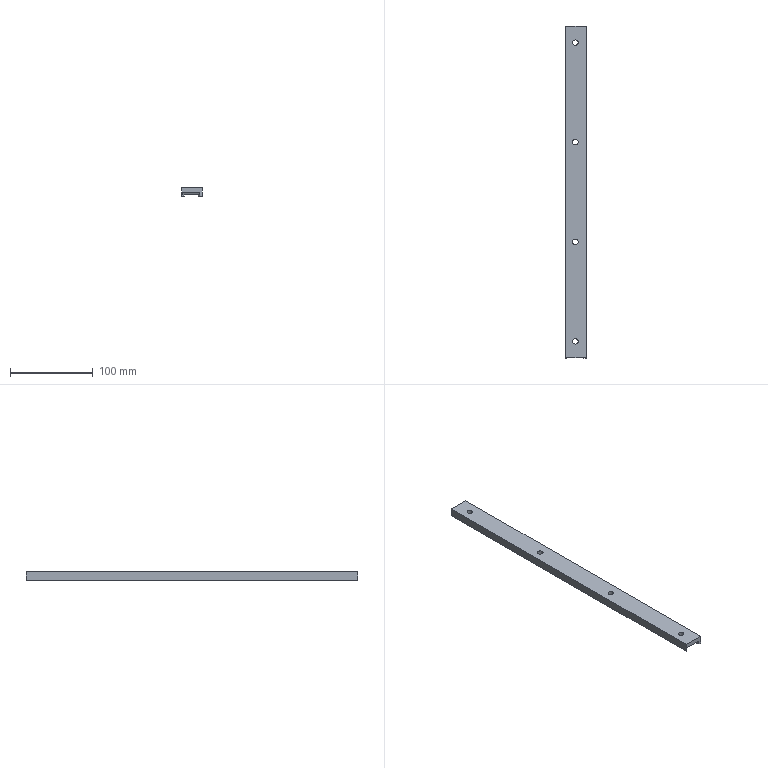Part | SolidWorks | features BaseBody 1 | 1 solid | 29 faces | box 24.5 x 400 x 10 mm | volume 79904 mm3 | plane 13 | cone 8 | cylinder 8 | commonest cylinder face diameters 6.6 x8
STEP:
#1=CARTESIAN_POINT('',(14.8,180.,-4.5));
#2=VERTEX_POINT('',#1);
#3=CARTESIAN_POINT('',(8.2,180.,-4.5));
#4=VERTEX_POINT('',#3);
#5=CARTESIAN_POINT('',(11.5,180.,-4.5));
#6=DIRECTION('',(0.,0.,-1.));
#7=DIRECTION('',(-1.,0.,0.));
#8=AXIS2_PLACEMENT_3D('',#5,#6,#7);
#9=CIRCLE('',#8,3.3);
#10=EDGE_CURVE('',#2,#4,#9,.T.);
#11=ORIENTED_EDGE('',*,*,#10,.F.);
#12=CARTESIAN_POINT('',(17.9,180.,-7.6));
#13=VERTEX_POINT('',#12);
#14=CARTESIAN_POINT('',(17.9,180.,-7.6));
#15=DIRECTION('',(0.7071,0.,-0.7071));
#16=VECTOR('',#15,1000.);
#17=LINE('',#14,#16);
#18=EDGE_CURVE('',#2,#13,#17,.T.);
#19=ORIENTED_EDGE('',*,*,#18,.T.);
#20=CARTESIAN_POINT('',(5.1,180.,-7.6));
#21=VERTEX_POINT('',#20);
#22=CARTESIAN_POINT('',(11.5,180.,-7.6));
#23=DIRECTION('',(0.,0.,-1.));
#24=DIRECTION('',(-1.,0.,0.));
#25=AXIS2_PLACEMENT_3D('',#22,#23,#24);
#26=CIRCLE('',#25,6.4);
#27=EDGE_CURVE('',#13,#21,#26,.T.);
#28=ORIENTED_EDGE('',*,*,#27,.T.);
#29=CARTESIAN_POINT('',(5.1,180.,-7.6));
#30=DIRECTION('',(-0.7071,0.,-0.7071));
#31=VECTOR('',#30,1000.);
#32=LINE('',#29,#31);
#33=EDGE_CURVE('',#4,#21,#32,.T.);
#34=ORIENTED_EDGE('',*,*,#33,.F.);
#35=EDGE_LOOP('',(#11,#19,#28,#34));
#36=FACE_OUTER_BOUND('',#35,.T.);
#37=CARTESIAN_POINT('',(11.5,180.,-7.6));
#38=DIRECTION('',(0.,0.,-1.));
#39=DIRECTION('',(-1.,0.,0.));
#40=AXIS2_PLACEMENT_3D('',#37,#38,#39);
#41=CONICAL_SURFACE('',#40,6.4,0.7854);
#42=ADVANCED_FACE('',(#36),#41,.F.);
#43=CARTESIAN_POINT('',(14.8,180.,0.));
#44=VERTEX_POINT('',#43);
#45=CARTESIAN_POINT('',(8.2,180.,0.));
#46=VERTEX_POINT('',#45);
#47=CARTESIAN_POINT('',(11.5,180.,0.));
#48=DIRECTION('',(0.,0.,-1.));
#49=DIRECTION('',(-1.,0.,0.));
#50=AXIS2_PLACEMENT_3D('',#47,#48,#49);
#51=CIRCLE('',#50,3.3);
#52=EDGE_CURVE('',#44,#46,#51,.T.);
#53=ORIENTED_EDGE('',*,*,#52,.F.);
#54=CARTESIAN_POINT('',(14.8,180.,-7.6));
#55=DIRECTION('',(0.,0.,-1.));
#56=VECTOR('',#55,1000.);
#57=LINE('',#54,#56);
#58=EDGE_CURVE('',#44,#2,#57,.T.);
#59=ORIENTED_EDGE('',*,*,#58,.T.);
#60=ORIENTED_EDGE('',*,*,#10,.T.);
#61=CARTESIAN_POINT('',(8.2,180.,-7.6));
#62=DIRECTION('',(0.,0.,-1.));
#63=VECTOR('',#62,1000.);
#64=LINE('',#61,#63);
#65=EDGE_CURVE('',#46,#4,#64,.T.);
#66=ORIENTED_EDGE('',*,*,#65,.F.);
#67=EDGE_LOOP('',(#53,#59,#60,#66));
#68=FACE_OUTER_BOUND('',#67,.T.);
#69=CARTESIAN_POINT('',(11.5,180.,-7.6));
#70=DIRECTION('',(0.,0.,-1.));
#71=DIRECTION('',(-1.,0.,0.));
#72=AXIS2_PLACEMENT_3D('',#69,#70,#71);
#73=CYLINDRICAL_SURFACE('',#72,3.3);
#74=ADVANCED_FACE('',(#68),#73,.F.);
#75=CARTESIAN_POINT('',(14.8,60.,-4.5));
#76=VERTEX_POINT('',#75);
#77=CARTESIAN_POINT('',(8.2,60.,-4.5));
#78=VERTEX_POINT('',#77);
#79=CARTESIAN_POINT('',(11.5,60.,-4.5));
#80=DIRECTION('',(0.,0.,-1.));
#81=DIRECTION('',(-1.,0.,0.));
#82=AXIS2_PLACEMENT_3D('',#79,#80,#81);
#83=CIRCLE('',#82,3.3);
#84=EDGE_CURVE('',#76,#78,#83,.T.);
#85=ORIENTED_EDGE('',*,*,#84,.F.);
#86=CARTESIAN_POINT('',(17.9,60.,-7.6));
#87=VERTEX_POINT('',#86);
#88=CARTESIAN_POINT('',(17.9,60.,-7.6));
#89=DIRECTION('',(0.7071,0.,-0.7071));
#90=VECTOR('',#89,1000.);
#91=LINE('',#88,#90);
#92=EDGE_CURVE('',#76,#87,#91,.T.);
#93=ORIENTED_EDGE('',*,*,#92,.T.);
#94=CARTESIAN_POINT('',(5.1,60.,-7.6));
#95=VERTEX_POINT('',#94);
#96=CARTESIAN_POINT('',(11.5,60.,-7.6));
#97=DIRECTION('',(0.,0.,-1.));
#98=DIRECTION('',(-1.,0.,0.));
#99=AXIS2_PLACEMENT_3D('',#96,#97,#98);
#100=CIRCLE('',#99,6.4);
#101=EDGE_CURVE('',#87,#95,#100,.T.);
#102=ORIENTED_EDGE('',*,*,#101,.T.);
#103=CARTESIAN_POINT('',(5.1,60.,-7.6));
#104=DIRECTION('',(-0.7071,0.,-0.7071));
#105=VECTOR('',#104,1000.);
#106=LINE('',#103,#105);
#107=EDGE_CURVE('',#78,#95,#106,.T.);
#108=ORIENTED_EDGE('',*,*,#107,.F.);
#109=EDGE_LOOP('',(#85,#93,#102,#108));
#110=FACE_OUTER_BOUND('',#109,.T.);
#111=CARTESIAN_POINT('',(11.5,60.,-7.6));
#112=DIRECTION('',(0.,0.,-1.));
#113=DIRECTION('',(-1.,0.,0.));
#114=AXIS2_PLACEMENT_3D('',#111,#112,#113);
#115=CONICAL_SURFACE('',#114,6.4,0.7854);
#116=ADVANCED_FACE('',(#110),#115,.F.);
#117=CARTESIAN_POINT('',(14.8,60.,0.));
#118=VERTEX_POINT('',#117);
#119=CARTESIAN_POINT('',(8.2,60.,0.));
#120=VERTEX_POINT('',#119);
#121=CARTESIAN_POINT('',(11.5,60.,0.));
#122=DIRECTION('',(0.,0.,-1.));
#123=DIRECTION('',(-1.,0.,0.));
#124=AXIS2_PLACEMENT_3D('',#121,#122,#123);
#125=CIRCLE('',#124,3.3);
#126=EDGE_CURVE('',#118,#120,#125,.T.);
#127=ORIENTED_EDGE('',*,*,#126,.F.);
#128=CARTESIAN_POINT('',(14.8,60.,-7.6));
#129=DIRECTION('',(0.,0.,-1.));
#130=VECTOR('',#129,1000.);
#131=LINE('',#128,#130);
#132=EDGE_CURVE('',#118,#76,#131,.T.);
#133=ORIENTED_EDGE('',*,*,#132,.T.);
#134=ORIENTED_EDGE('',*,*,#84,.T.);
#135=CARTESIAN_POINT('',(8.2,60.,-7.6));
#136=DIRECTION('',(0.,0.,-1.));
#137=VECTOR('',#136,1000.);
#138=LINE('',#135,#137);
#139=EDGE_CURVE('',#120,#78,#138,.T.);
#140=ORIENTED_EDGE('',*,*,#139,.F.);
#141=EDGE_LOOP('',(#127,#133,#134,#140));
#142=FACE_OUTER_BOUND('',#141,.T.);
#143=CARTESIAN_POINT('',(11.5,60.,-7.6));
#144=DIRECTION('',(0.,0.,-1.));
#145=DIRECTION('',(-1.,0.,0.));
#146=AXIS2_PLACEMENT_3D('',#143,#144,#145);
#147=CYLINDRICAL_SURFACE('',#146,3.3);
#148=ADVANCED_FACE('',(#142),#147,.F.);
#149=CARTESIAN_POINT('',(14.8,-60.,-4.5));
#150=VERTEX_POINT('',#149);
#151=CARTESIAN_POINT('',(8.2,-60.,-4.5));
#152=VERTEX_POINT('',#151);
#153=CARTESIAN_POINT('',(11.5,-60.,-4.5));
#154=DIRECTION('',(0.,0.,-1.));
#155=DIRECTION('',(-1.,0.,0.));
#156=AXIS2_PLACEMENT_3D('',#153,#154,#155);
#157=CIRCLE('',#156,3.3);
#158=EDGE_CURVE('',#150,#152,#157,.T.);
#159=ORIENTED_EDGE('',*,*,#158,.F.);
#160=CARTESIAN_POINT('',(17.9,-60.,-7.6));
#161=VERTEX_POINT('',#160);
#162=CARTESIAN_POINT('',(17.9,-60.,-7.6));
#163=DIRECTION('',(0.7071,0.,-0.7071));
#164=VECTOR('',#163,1000.);
#165=LINE('',#162,#164);
#166=EDGE_CURVE('',#150,#161,#165,.T.);
#167=ORIENTED_EDGE('',*,*,#166,.T.);
#168=CARTESIAN_POINT('',(5.1,-60.,-7.6));
#169=VERTEX_POINT('',#168);
#170=CARTESIAN_POINT('',(11.5,-60.,-7.6));
#171=DIRECTION('',(0.,0.,-1.));
#172=DIRECTION('',(-1.,0.,0.));
#173=AXIS2_PLACEMENT_3D('',#170,#171,#172);
#174=CIRCLE('',#173,6.4);
#175=EDGE_CURVE('',#161,#169,#174,.T.);
#176=ORIENTED_EDGE('',*,*,#175,.T.);
#177=CARTESIAN_POINT('',(5.1,-60.,-7.6));
#178=DIRECTION('',(-0.7071,0.,-0.7071));
#179=VECTOR('',#178,1000.);
#180=LINE('',#177,#179);
#181=EDGE_CURVE('',#152,#169,#180,.T.);
#182=ORIENTED_EDGE('',*,*,#181,.F.);
#183=EDGE_LOOP('',(#159,#167,#176,#182));
#184=FACE_OUTER_BOUND('',#183,.T.);
#185=CARTESIAN_POINT('',(11.5,-60.,-7.6));
#186=DIRECTION('',(0.,0.,-1.));
#187=DIRECTION('',(-1.,0.,0.));
#188=AXIS2_PLACEMENT_3D('',#185,#186,#187);
#189=CONICAL_SURFACE('',#188,6.4,0.7854);
#190=ADVANCED_FACE('',(#184),#189,.F.);
#191=CARTESIAN_POINT('',(14.8,-60.,0.));
#192=VERTEX_POINT('',#191);
#193=CARTESIAN_POINT('',(8.2,-60.,0.));
#194=VERTEX_POINT('',#193);
#195=CARTESIAN_POINT('',(11.5,-60.,0.));
#196=DIRECTION('',(0.,0.,-1.));
#197=DIRECTION('',(-1.,0.,0.));
#198=AXIS2_PLACEMENT_3D('',#195,#196,#197);
#199=CIRCLE('',#198,3.3);
#200=EDGE_CURVE('',#192,#194,#199,.T.);
#201=ORIENTED_EDGE('',*,*,#200,.F.);
#202=CARTESIAN_POINT('',(14.8,-60.,-7.6));
#203=DIRECTION('',(0.,0.,-1.));
#204=VECTOR('',#203,1000.);
#205=LINE('',#202,#204);
#206=EDGE_CURVE('',#192,#150,#205,.T.);
#207=ORIENTED_EDGE('',*,*,#206,.T.);
#208=ORIENTED_EDGE('',*,*,#158,.T.);
#209=CARTESIAN_POINT('',(8.2,-60.,-7.6));
#210=DIRECTION('',(0.,0.,-1.));
#211=VECTOR('',#210,1000.);
#212=LINE('',#209,#211);
#213=EDGE_CURVE('',#194,#152,#212,.T.);
#214=ORIENTED_EDGE('',*,*,#213,.F.);
#215=EDGE_LOOP('',(#201,#207,#208,#214));
#216=FACE_OUTER_BOUND('',#215,.T.);
#217=CARTESIAN_POINT('',(11.5,-60.,-7.6));
#218=DIRECTION('',(0.,0.,-1.));
#219=DIRECTION('',(-1.,0.,0.));
#220=AXIS2_PLACEMENT_3D('',#217,#218,#219);
#221=CYLINDRICAL_SURFACE('',#220,3.3);
#222=ADVANCED_FACE('',(#216),#221,.F.);
#223=CARTESIAN_POINT('',(14.8,-180.,-4.5));
#224=VERTEX_POINT('',#223);
#225=CARTESIAN_POINT('',(8.2,-180.,-4.5));
#226=VERTEX_POINT('',#225);
#227=CARTESIAN_POINT('',(11.5,-180.,-4.5));
#228=DIRECTION('',(0.,0.,-1.));
#229=DIRECTION('',(-1.,0.,0.));
#230=AXIS2_PLACEMENT_3D('',#227,#228,#229);
#231=CIRCLE('',#230,3.3);
#232=EDGE_CURVE('',#224,#226,#231,.T.);
#233=ORIENTED_EDGE('',*,*,#232,.F.);
#234=CARTESIAN_POINT('',(17.9,-180.,-7.6));
#235=VERTEX_POINT('',#234);
#236=CARTESIAN_POINT('',(17.9,-180.,-7.6));
#237=DIRECTION('',(0.7071,0.,-0.7071));
#238=VECTOR('',#237,1000.);
#239=LINE('',#236,#238);
#240=EDGE_CURVE('',#224,#235,#239,.T.);
#241=ORIENTED_EDGE('',*,*,#240,.T.);
#242=CARTESIAN_POINT('',(5.1,-180.,-7.6));
#243=VERTEX_POINT('',#242);
#244=CARTESIAN_POINT('',(11.5,-180.,-7.6));
#245=DIRECTION('',(0.,0.,-1.));
#246=DIRECTION('',(-1.,0.,0.));
#247=AXIS2_PLACEMENT_3D('',#244,#245,#246);
#248=CIRCLE('',#247,6.4);
#249=EDGE_CURVE('',#235,#243,#248,.T.);
#250=ORIENTED_EDGE('',*,*,#249,.T.);
#251=CARTESIAN_POINT('',(5.1,-180.,-7.6));
#252=DIRECTION('',(-0.7071,0.,-0.7071));
#253=VECTOR('',#252,1000.);
#254=LINE('',#251,#253);
#255=EDGE_CURVE('',#226,#243,#254,.T.);
#256=ORIENTED_EDGE('',*,*,#255,.F.);
#257=EDGE_LOOP('',(#233,#241,#250,#256));
#258=FACE_OUTER_BOUND('',#257,.T.);
#259=CARTESIAN_POINT('',(11.5,-180.,-7.6));
#260=DIRECTION('',(0.,0.,-1.));
#261=DIRECTION('',(-1.,0.,0.));
#262=AXIS2_PLACEMENT_3D('',#259,#260,#261);
#263=CONICAL_SURFACE('',#262,6.4,0.7854);
#264=ADVANCED_FACE('',(#258),#263,.F.);
#265=CARTESIAN_POINT('',(14.8,-180.,0.));
#266=VERTEX_POINT('',#265);
#267=CARTESIAN_POINT('',(8.2,-180.,0.));
#268=VERTEX_POINT('',#267);
#269=CARTESIAN_POINT('',(11.5,-180.,0.));
#270=DIRECTION('',(0.,0.,-1.));
#271=DIRECTION('',(-1.,0.,0.));
#272=AXIS2_PLACEMENT_3D('',#269,#270,#271);
#273=CIRCLE('',#272,3.3);
#274=EDGE_CURVE('',#266,#268,#273,.T.);
#275=ORIENTED_EDGE('',*,*,#274,.F.);
#276=CARTESIAN_POINT('',(14.8,-180.,-7.6));
#277=DIRECTION('',(0.,0.,-1.));
#278=VECTOR('',#277,1000.);
#279=LINE('',#276,#278);
#280=EDGE_CURVE('',#266,#224,#279,.T.);
#281=ORIENTED_EDGE('',*,*,#280,.T.);
#282=ORIENTED_EDGE('',*,*,#232,.T.);
#283=CARTESIAN_POINT('',(8.2,-180.,-7.6));
#284=DIRECTION('',(0.,0.,-1.));
#285=VECTOR('',#284,1000.);
#286=LINE('',#283,#285);
#287=EDGE_CURVE('',#268,#226,#286,.T.);
#288=ORIENTED_EDGE('',*,*,#287,.F.);
#289=EDGE_LOOP('',(#275,#281,#282,#288));
#290=FACE_OUTER_BOUND('',#289,.T.);
#291=CARTESIAN_POINT('',(11.5,-180.,-7.6));
#292=DIRECTION('',(0.,0.,-1.));
#293=DIRECTION('',(-1.,0.,0.));
#294=AXIS2_PLACEMENT_3D('',#291,#292,#293);
#295=CYLINDRICAL_SURFACE('',#294,3.3);
#296=ADVANCED_FACE('',(#290),#295,.F.);
#297=CARTESIAN_POINT('',(1.237,-200.,-5.837));
#298=VERTEX_POINT('',#297);
#299=CARTESIAN_POINT('',(3.,-190.,-7.6));
#300=VERTEX_POINT('',#299);
#301=CARTESIAN_POINT('',(3.07,-189.602,-7.67));
#302=DIRECTION('',(0.1711,0.9703,-0.1711));
#303=VECTOR('',#302,1000.);
#304=LINE('',#301,#303);
#305=EDGE_CURVE('',#298,#300,#304,.T.);
#306=ORIENTED_EDGE('',*,*,#305,.F.);
#307=CARTESIAN_POINT('',(1.237,-200.,-10.));
#308=VERTEX_POINT('',#307);
#309=CARTESIAN_POINT('',(1.237,-200.,-5.837));
#310=DIRECTION('',(0.,0.,1.));
#311=VECTOR('',#310,1000.);
#312=LINE('',#309,#311);
#313=EDGE_CURVE('',#308,#298,#312,.T.);
#314=ORIENTED_EDGE('',*,*,#313,.F.);
#315=CARTESIAN_POINT('',(3.,-190.,-10.));
#316=VERTEX_POINT('',#315);
#317=CARTESIAN_POINT('',(3.,-190.,-10.));
#318=DIRECTION('',(-0.1736,-0.9848,0.));
#319=VECTOR('',#318,1000.);
#320=LINE('',#317,#319);
#321=EDGE_CURVE('',#316,#308,#320,.T.);
#322=ORIENTED_EDGE('',*,*,#321,.F.);
#323=CARTESIAN_POINT('',(3.,-190.,-10.));
#324=DIRECTION('',(0.,0.,-1.));
#325=VECTOR('',#324,1000.);
#326=LINE('',#323,#325);
#327=EDGE_CURVE('',#300,#316,#326,.T.);
#328=ORIENTED_EDGE('',*,*,#327,.F.);
#329=EDGE_LOOP('',(#306,#314,#322,#328));
#330=FACE_OUTER_BOUND('',#329,.T.);
#331=CARTESIAN_POINT('',(3.,-190.,-10.));
#332=DIRECTION('',(0.9848,-0.1736,0.));
#333=DIRECTION('',(0.,0.,-1.));
#334=AXIS2_PLACEMENT_3D('',#331,#332,#333);
#335=PLANE('',#334);
#336=ADVANCED_FACE('',(#330),#335,.T.);
#337=CARTESIAN_POINT('',(21.763,-200.,-10.));
#338=VERTEX_POINT('',#337);
#339=CARTESIAN_POINT('',(20.,-190.,-10.));
#340=VERTEX_POINT('',#339);
#341=CARTESIAN_POINT('',(20.,-190.,-10.));
#342=DIRECTION('',(-0.1736,0.9848,0.));
#343=VECTOR('',#342,1000.);
#344=LINE('',#341,#343);
#345=EDGE_CURVE('',#338,#340,#344,.T.);
#346=ORIENTED_EDGE('',*,*,#345,.F.);
#347=CARTESIAN_POINT('',(21.763,-200.,-5.837));
#348=VERTEX_POINT('',#347);
#349=CARTESIAN_POINT('',(21.763,-200.,-10.));
#350=DIRECTION('',(0.,0.,-1.));
#351=VECTOR('',#350,1000.);
#352=LINE('',#349,#351);
#353=EDGE_CURVE('',#348,#338,#352,.T.);
#354=ORIENTED_EDGE('',*,*,#353,.F.);
#355=CARTESIAN_POINT('',(20.,-190.,-7.6));
#356=VERTEX_POINT('',#355);
#357=CARTESIAN_POINT('',(19.93,-189.602,-7.67));
#358=DIRECTION('',(0.1711,-0.9703,0.1711));
#359=VECTOR('',#358,1000.);
#360=LINE('',#357,#359);
#361=EDGE_CURVE('',#356,#348,#360,.T.);
#362=ORIENTED_EDGE('',*,*,#361,.F.);
#363=CARTESIAN_POINT('',(20.,-190.,-5.837));
#364=DIRECTION('',(0.,0.,1.));
#365=VECTOR('',#364,1000.);
#366=LINE('',#363,#365);
#367=EDGE_CURVE('',#340,#356,#366,.T.);
#368=ORIENTED_EDGE('',*,*,#367,.F.);
#369=EDGE_LOOP('',(#346,#354,#362,#368));
#370=FACE_OUTER_BOUND('',#369,.T.);
#371=CARTESIAN_POINT('',(20.,-190.,-10.));
#372=DIRECTION('',(-0.9848,-0.1736,0.));
#373=DIRECTION('',(-0.1736,0.9848,0.));
#374=AXIS2_PLACEMENT_3D('',#371,#372,#373);
#375=PLANE('',#374);
#376=ADVANCED_FACE('',(#370),#375,.T.);
#377=CARTESIAN_POINT('',(3.,-190.,-7.6));
#378=DIRECTION('',(-1.,0.,0.));
#379=VECTOR('',#378,1000.);
#380=LINE('',#377,#379);
#381=EDGE_CURVE('',#356,#300,#380,.T.);
#382=ORIENTED_EDGE('',*,*,#381,.F.);
#383=ORIENTED_EDGE('',*,*,#361,.T.);
#384=CARTESIAN_POINT('',(20.,-200.,-5.837));
#385=DIRECTION('',(1.,0.,0.));
#386=VECTOR('',#385,1000.);
#387=LINE('',#384,#386);
#388=EDGE_CURVE('',#298,#348,#387,.T.);
#389=ORIENTED_EDGE('',*,*,#388,.F.);
#390=ORIENTED_EDGE('',*,*,#305,.T.);
#391=EDGE_LOOP('',(#382,#383,#389,#390));
#392=FACE_OUTER_BOUND('',#391,.T.);
#393=CARTESIAN_POINT('',(3.,-190.,-7.6));
#394=DIRECTION('',(0.,-0.1736,-0.9848));
#395=DIRECTION('',(0.,-0.9848,0.1736));
#396=AXIS2_PLACEMENT_3D('',#393,#394,#395);
#397=PLANE('',#396);
#398=ADVANCED_FACE('',(#392),#397,.T.);
#399=ORIENTED_EDGE('',*,*,#388,.T.);
#400=ORIENTED_EDGE('',*,*,#353,.T.);
#401=CARTESIAN_POINT('',(24.5,-200.,-10.));
#402=VERTEX_POINT('',#401);
#403=CARTESIAN_POINT('',(20.,-200.,-10.));
#404=DIRECTION('',(-1.,0.,0.));
#405=VECTOR('',#404,1000.);
#406=LINE('',#403,#405);
#407=EDGE_CURVE('',#402,#338,#406,.T.);
#408=ORIENTED_EDGE('',*,*,#407,.F.);
#409=CARTESIAN_POINT('',(24.5,-200.,0.));
#410=VERTEX_POINT('',#409);
#411=CARTESIAN_POINT('',(24.5,-200.,-10.));
#412=DIRECTION('',(0.,0.,-1.));
#413=VECTOR('',#412,1000.);
#414=LINE('',#411,#413);
#415=EDGE_CURVE('',#410,#402,#414,.T.);
#416=ORIENTED_EDGE('',*,*,#415,.F.);
#417=CARTESIAN_POINT('',(0.,-200.,0.));
#418=VERTEX_POINT('',#417);
#419=CARTESIAN_POINT('',(24.5,-200.,0.));
#420=DIRECTION('',(1.,0.,0.));
#421=VECTOR('',#420,1000.);
#422=LINE('',#419,#421);
#423=EDGE_CURVE('',#418,#410,#422,.T.);
#424=ORIENTED_EDGE('',*,*,#423,.F.);
#425=CARTESIAN_POINT('',(0.,-200.,-10.));
#426=VERTEX_POINT('',#425);
#427=CARTESIAN_POINT('',(0.,-200.,0.));
#428=DIRECTION('',(0.,0.,1.));
#429=VECTOR('',#428,1000.);
#430=LINE('',#427,#429);
#431=EDGE_CURVE('',#426,#418,#430,.T.);
#432=ORIENTED_EDGE('',*,*,#431,.F.);
#433=CARTESIAN_POINT('',(0.,-200.,-10.));
#434=DIRECTION('',(-1.,0.,0.));
#435=VECTOR('',#434,1000.);
#436=LINE('',#433,#435);
#437=EDGE_CURVE('',#308,#426,#436,.T.);
#438=ORIENTED_EDGE('',*,*,#437,.F.);
#439=ORIENTED_EDGE('',*,*,#313,.T.);
#440=EDGE_LOOP('',(#399,#400,#408,#416,#424,#432,#438,#439));
#441=FACE_OUTER_BOUND('',#440,.T.);
#442=CARTESIAN_POINT('',(0.,-200.,0.));
#443=DIRECTION('',(0.,-1.,0.));
#444=DIRECTION('',(0.,0.,-1.));
#445=AXIS2_PLACEMENT_3D('',#442,#443,#444);
#446=PLANE('',#445);
#447=ADVANCED_FACE('',(#441),#446,.T.);
#448=CARTESIAN_POINT('',(0.,200.,0.));
#449=VERTEX_POINT('',#448);
#450=CARTESIAN_POINT('',(24.5,200.,0.));
#451=VERTEX_POINT('',#450);
#452=CARTESIAN_POINT('',(24.5,200.,0.));
#453=DIRECTION('',(1.,0.,0.));
#454=VECTOR('',#453,1000.);
#455=LINE('',#452,#454);
#456=EDGE_CURVE('',#449,#451,#455,.T.);
#457=ORIENTED_EDGE('',*,*,#456,.T.);
#458=CARTESIAN_POINT('',(24.5,200.,-10.));
#459=VERTEX_POINT('',#458);
#460=CARTESIAN_POINT('',(24.5,200.,-10.));
#461=DIRECTION('',(0.,0.,-1.));
#462=VECTOR('',#461,1000.);
#463=LINE('',#460,#462);
#464=EDGE_CURVE('',#451,#459,#463,.T.);
#465=ORIENTED_EDGE('',*,*,#464,.T.);
#466=CARTESIAN_POINT('',(20.,200.,-10.));
#467=VERTEX_POINT('',#466);
#468=CARTESIAN_POINT('',(20.,200.,-10.));
#469=DIRECTION('',(-1.,0.,0.));
#470=VECTOR('',#469,1000.);
#471=LINE('',#468,#470);
#472=EDGE_CURVE('',#459,#467,#471,.T.);
#473=ORIENTED_EDGE('',*,*,#472,.T.);
#474=CARTESIAN_POINT('',(20.,200.,-7.6));
#475=VERTEX_POINT('',#474);
#476=CARTESIAN_POINT('',(20.,200.,-10.));
#477=DIRECTION('',(0.,0.,1.));
#478=VECTOR('',#477,1000.);
#479=LINE('',#476,#478);
#480=EDGE_CURVE('',#467,#475,#479,.T.);
#481=ORIENTED_EDGE('',*,*,#480,.T.);
#482=CARTESIAN_POINT('',(3.,200.,-7.6));
#483=VERTEX_POINT('',#482);
#484=CARTESIAN_POINT('',(3.,200.,-7.6));
#485=DIRECTION('',(-1.,0.,0.));
#486=VECTOR('',#485,1000.);
#487=LINE('',#484,#486);
#488=EDGE_CURVE('',#475,#483,#487,.T.);
#489=ORIENTED_EDGE('',*,*,#488,.T.);
#490=CARTESIAN_POINT('',(3.,200.,-10.));
#491=VERTEX_POINT('',#490);
#492=CARTESIAN_POINT('',(3.,200.,-10.));
#493=DIRECTION('',(0.,0.,-1.));
#494=VECTOR('',#493,1000.);
#495=LINE('',#492,#494);
#496=EDGE_CURVE('',#483,#491,#495,.T.);
#497=ORIENTED_EDGE('',*,*,#496,.T.);
#498=CARTESIAN_POINT('',(0.,200.,-10.));
#499=VERTEX_POINT('',#498);
#500=CARTESIAN_POINT('',(0.,200.,-10.));
#501=DIRECTION('',(-1.,0.,0.));
#502=VECTOR('',#501,1000.);
#503=LINE('',#500,#502);
#504=EDGE_CURVE('',#491,#499,#503,.T.);
#505=ORIENTED_EDGE('',*,*,#504,.T.);
#506=CARTESIAN_POINT('',(0.,200.,0.));
#507=DIRECTION('',(0.,0.,1.));
#508=VECTOR('',#507,1000.);
#509=LINE('',#506,#508);
#510=EDGE_CURVE('',#499,#449,#509,.T.);
#511=ORIENTED_EDGE('',*,*,#510,.T.);
#512=EDGE_LOOP('',(#457,#465,#473,#481,#489,#497,#505,#511));
#513=FACE_OUTER_BOUND('',#512,.T.);
#514=CARTESIAN_POINT('',(0.,200.,0.));
#515=DIRECTION('',(0.,-1.,0.));
#516=DIRECTION('',(0.,0.,-1.));
#517=AXIS2_PLACEMENT_3D('',#514,#515,#516);
#518=PLANE('',#517);
#519=ADVANCED_FACE('',(#513),#518,.F.);
#520=ORIENTED_EDGE('',*,*,#431,.T.);
#521=CARTESIAN_POINT('',(0.,200.,0.));
#522=DIRECTION('',(0.,-1.,0.));
#523=VECTOR('',#522,1000.);
#524=LINE('',#521,#523);
#525=EDGE_CURVE('',#449,#418,#524,.T.);
#526=ORIENTED_EDGE('',*,*,#525,.F.);
#527=ORIENTED_EDGE('',*,*,#510,.F.);
#528=CARTESIAN_POINT('',(0.,200.,-10.));
#529=DIRECTION('',(0.,-1.,0.));
#530=VECTOR('',#529,1000.);
#531=LINE('',#528,#530);
#532=EDGE_CURVE('',#499,#426,#531,.T.);
#533=ORIENTED_EDGE('',*,*,#532,.T.);
#534=EDGE_LOOP('',(#520,#526,#527,#533));
#535=FACE_OUTER_BOUND('',#534,.T.);
#536=CARTESIAN_POINT('',(0.,200.,0.));
#537=DIRECTION('',(1.,0.,0.));
#538=DIRECTION('',(0.,1.,0.));
#539=AXIS2_PLACEMENT_3D('',#536,#537,#538);
#540=PLANE('',#539);
#541=ADVANCED_FACE('',(#535),#540,.F.);
#542=CARTESIAN_POINT('',(3.,200.,-10.));
#543=DIRECTION('',(0.,-1.,0.));
#544=VECTOR('',#543,1000.);
#545=LINE('',#542,#544);
#546=EDGE_CURVE('',#491,#316,#545,.T.);
#547=ORIENTED_EDGE('',*,*,#546,.T.);
#548=ORIENTED_EDGE('',*,*,#321,.T.);
#549=ORIENTED_EDGE('',*,*,#437,.T.);
#550=ORIENTED_EDGE('',*,*,#532,.F.);
#551=ORIENTED_EDGE('',*,*,#504,.F.);
#552=EDGE_LOOP('',(#547,#548,#549,#550,#551));
#553=FACE_OUTER_BOUND('',#552,.T.);
#554=CARTESIAN_POINT('',(0.,200.,-10.));
#555=DIRECTION('',(0.,0.,1.));
#556=DIRECTION('',(1.,0.,0.));
#557=AXIS2_PLACEMENT_3D('',#554,#555,#556);
#558=PLANE('',#557);
#559=ADVANCED_FACE('',(#553),#558,.F.);
#560=CARTESIAN_POINT('',(3.,200.,-7.6));
#561=DIRECTION('',(0.,-1.,0.));
#562=VECTOR('',#561,1000.);
#563=LINE('',#560,#562);
#564=EDGE_CURVE('',#483,#300,#563,.T.);
#565=ORIENTED_EDGE('',*,*,#564,.T.);
#566=ORIENTED_EDGE('',*,*,#327,.T.);
#567=ORIENTED_EDGE('',*,*,#546,.F.);
#568=ORIENTED_EDGE('',*,*,#496,.F.);
#569=EDGE_LOOP('',(#565,#566,#567,#568));
#570=FACE_OUTER_BOUND('',#569,.T.);
#571=CARTESIAN_POINT('',(3.,200.,-10.));
#572=DIRECTION('',(-1.,0.,0.));
#573=DIRECTION('',(0.,0.,1.));
#574=AXIS2_PLACEMENT_3D('',#571,#572,#573);
#575=PLANE('',#574);
#576=ADVANCED_FACE('',(#570),#575,.F.);
#577=CARTESIAN_POINT('',(20.,200.,-10.));
#578=DIRECTION('',(0.,-1.,0.));
#579=VECTOR('',#578,1000.);
#580=LINE('',#577,#579);
#581=EDGE_CURVE('',#467,#340,#580,.T.);
#582=ORIENTED_EDGE('',*,*,#581,.T.);
#583=ORIENTED_EDGE('',*,*,#367,.T.);
#584=CARTESIAN_POINT('',(20.,200.,-7.6));
#585=DIRECTION('',(0.,-1.,0.));
#586=VECTOR('',#585,1000.);
#587=LINE('',#584,#586);
#588=EDGE_CURVE('',#475,#356,#587,.T.);
#589=ORIENTED_EDGE('',*,*,#588,.F.);
#590=ORIENTED_EDGE('',*,*,#480,.F.);
#591=EDGE_LOOP('',(#582,#583,#589,#590));
#592=FACE_OUTER_BOUND('',#591,.T.);
#593=CARTESIAN_POINT('',(20.,200.,-10.));
#594=DIRECTION('',(1.,0.,0.));
#595=DIRECTION('',(0.,1.,0.));
#596=AXIS2_PLACEMENT_3D('',#593,#594,#595);
#597=PLANE('',#596);
#598=ADVANCED_FACE('',(#592),#597,.F.);
#599=ORIENTED_EDGE('',*,*,#407,.T.);
#600=ORIENTED_EDGE('',*,*,#345,.T.);
#601=ORIENTED_EDGE('',*,*,#581,.F.);
#602=ORIENTED_EDGE('',*,*,#472,.F.);
#603=CARTESIAN_POINT('',(24.5,200.,-10.));
#604=DIRECTION('',(0.,-1.,0.));
#605=VECTOR('',#604,1000.);
#606=LINE('',#603,#605);
#607=EDGE_CURVE('',#459,#402,#606,.T.);
#608=ORIENTED_EDGE('',*,*,#607,.T.);
#609=EDGE_LOOP('',(#599,#600,#601,#602,#608));
#610=FACE_OUTER_BOUND('',#609,.T.);
#611=CARTESIAN_POINT('',(20.,200.,-10.));
#612=DIRECTION('',(0.,0.,1.));
#613=DIRECTION('',(1.,0.,0.));
#614=AXIS2_PLACEMENT_3D('',#611,#612,#613);
#615=PLANE('',#614);
#616=ADVANCED_FACE('',(#610),#615,.F.);
#617=ORIENTED_EDGE('',*,*,#415,.T.);
#618=ORIENTED_EDGE('',*,*,#607,.F.);
#619=ORIENTED_EDGE('',*,*,#464,.F.);
#620=CARTESIAN_POINT('',(24.5,200.,0.));
#621=DIRECTION('',(0.,-1.,0.));
#622=VECTOR('',#621,1000.);
#623=LINE('',#620,#622);
#624=EDGE_CURVE('',#451,#410,#623,.T.);
#625=ORIENTED_EDGE('',*,*,#624,.T.);
#626=EDGE_LOOP('',(#617,#618,#619,#625));
#627=FACE_OUTER_BOUND('',#626,.T.);
#628=CARTESIAN_POINT('',(24.5,200.,-10.));
#629=DIRECTION('',(-1.,0.,0.));
#630=DIRECTION('',(0.,0.,1.));
#631=AXIS2_PLACEMENT_3D('',#628,#629,#630);
#632=PLANE('',#631);
#633=ADVANCED_FACE('',(#627),#632,.F.);
#634=CARTESIAN_POINT('',(11.5,-180.,0.));
#635=DIRECTION('',(0.,0.,-1.));
#636=DIRECTION('',(-1.,0.,0.));
#637=AXIS2_PLACEMENT_3D('',#634,#635,#636);
#638=CIRCLE('',#637,3.3);
#639=EDGE_CURVE('',#268,#266,#638,.T.);
#640=ORIENTED_EDGE('',*,*,#639,.T.);
#641=ORIENTED_EDGE('',*,*,#274,.T.);
#642=EDGE_LOOP('',(#640,#641));
#643=FACE_BOUND('',#642,.T.);
#644=CARTESIAN_POINT('',(11.5,-60.,0.));
#645=DIRECTION('',(0.,0.,-1.));
#646=DIRECTION('',(-1.,0.,0.));
#647=AXIS2_PLACEMENT_3D('',#644,#645,#646);
#648=CIRCLE('',#647,3.3);
#649=EDGE_CURVE('',#194,#192,#648,.T.);
#650=ORIENTED_EDGE('',*,*,#649,.T.);
#651=ORIENTED_EDGE('',*,*,#200,.T.);
#652=EDGE_LOOP('',(#650,#651));
#653=FACE_BOUND('',#652,.T.);
#654=CARTESIAN_POINT('',(11.5,60.,0.));
#655=DIRECTION('',(0.,0.,-1.));
#656=DIRECTION('',(-1.,0.,0.));
#657=AXIS2_PLACEMENT_3D('',#654,#655,#656);
#658=CIRCLE('',#657,3.3);
#659=EDGE_CURVE('',#120,#118,#658,.T.);
#660=ORIENTED_EDGE('',*,*,#659,.T.);
#661=ORIENTED_EDGE('',*,*,#126,.T.);
#662=EDGE_LOOP('',(#660,#661));
#663=FACE_BOUND('',#662,.T.);
#664=CARTESIAN_POINT('',(11.5,180.,0.));
#665=DIRECTION('',(0.,0.,-1.));
#666=DIRECTION('',(-1.,0.,0.));
#667=AXIS2_PLACEMENT_3D('',#664,#665,#666);
#668=CIRCLE('',#667,3.3);
#669=EDGE_CURVE('',#46,#44,#668,.T.);
#670=ORIENTED_EDGE('',*,*,#669,.T.);
#671=ORIENTED_EDGE('',*,*,#52,.T.);
#672=EDGE_LOOP('',(#670,#671));
#673=FACE_BOUND('',#672,.T.);
#674=ORIENTED_EDGE('',*,*,#423,.T.);
#675=ORIENTED_EDGE('',*,*,#624,.F.);
#676=ORIENTED_EDGE('',*,*,#456,.F.);
#677=ORIENTED_EDGE('',*,*,#525,.T.);
#678=EDGE_LOOP('',(#674,#675,#676,#677));
#679=FACE_OUTER_BOUND('',#678,.T.);
#680=CARTESIAN_POINT('',(24.5,200.,0.));
#681=DIRECTION('',(0.,0.,-1.));
#682=DIRECTION('',(-1.,0.,0.));
#683=AXIS2_PLACEMENT_3D('',#680,#681,#682);
#684=PLANE('',#683);
#685=ADVANCED_FACE('',(#643,#653,#663,#673,#679),#684,.F.);
#686=CARTESIAN_POINT('',(11.5,-60.,-7.6));
#687=DIRECTION('',(0.,0.,-1.));
#688=DIRECTION('',(-1.,0.,0.));
#689=AXIS2_PLACEMENT_3D('',#686,#687,#688);
#690=CIRCLE('',#689,6.4);
#691=EDGE_CURVE('',#169,#161,#690,.T.);
#692=ORIENTED_EDGE('',*,*,#691,.F.);
#693=ORIENTED_EDGE('',*,*,#175,.F.);
#694=EDGE_LOOP('',(#692,#693));
#695=FACE_BOUND('',#694,.T.);
#696=CARTESIAN_POINT('',(11.5,-180.,-7.6));
#697=DIRECTION('',(0.,0.,-1.));
#698=DIRECTION('',(-1.,0.,0.));
#699=AXIS2_PLACEMENT_3D('',#696,#697,#698);
#700=CIRCLE('',#699,6.4);
#701=EDGE_CURVE('',#243,#235,#700,.T.);
#702=ORIENTED_EDGE('',*,*,#701,.F.);
#703=ORIENTED_EDGE('',*,*,#249,.F.);
#704=EDGE_LOOP('',(#702,#703));
#705=FACE_BOUND('',#704,.T.);
#706=CARTESIAN_POINT('',(11.5,60.,-7.6));
#707=DIRECTION('',(0.,0.,-1.));
#708=DIRECTION('',(-1.,0.,0.));
#709=AXIS2_PLACEMENT_3D('',#706,#707,#708);
#710=CIRCLE('',#709,6.4);
#711=EDGE_CURVE('',#95,#87,#710,.T.);
#712=ORIENTED_EDGE('',*,*,#711,.F.);
#713=ORIENTED_EDGE('',*,*,#101,.F.);
#714=EDGE_LOOP('',(#712,#713));
#715=FACE_BOUND('',#714,.T.);
#716=CARTESIAN_POINT('',(11.5,180.,-7.6));
#717=DIRECTION('',(0.,0.,-1.));
#718=DIRECTION('',(-1.,0.,0.));
#719=AXIS2_PLACEMENT_3D('',#716,#717,#718);
#720=CIRCLE('',#719,6.4);
#721=EDGE_CURVE('',#21,#13,#720,.T.);
#722=ORIENTED_EDGE('',*,*,#721,.F.);
#723=ORIENTED_EDGE('',*,*,#27,.F.);
#724=EDGE_LOOP('',(#722,#723));
#725=FACE_BOUND('',#724,.T.);
#726=ORIENTED_EDGE('',*,*,#588,.T.);
#727=ORIENTED_EDGE('',*,*,#381,.T.);
#728=ORIENTED_EDGE('',*,*,#564,.F.);
#729=ORIENTED_EDGE('',*,*,#488,.F.);
#730=EDGE_LOOP('',(#726,#727,#728,#729));
#731=FACE_OUTER_BOUND('',#730,.T.);
#732=CARTESIAN_POINT('',(3.,200.,-7.6));
#733=DIRECTION('',(0.,0.,1.));
#734=DIRECTION('',(1.,0.,0.));
#735=AXIS2_PLACEMENT_3D('',#732,#733,#734);
#736=PLANE('',#735);
#737=ADVANCED_FACE('',(#695,#705,#715,#725,#731),#736,.F.);
#738=ORIENTED_EDGE('',*,*,#280,.F.);
#739=ORIENTED_EDGE('',*,*,#639,.F.);
#740=ORIENTED_EDGE('',*,*,#287,.T.);
#741=CARTESIAN_POINT('',(11.5,-180.,-4.5));
#742=DIRECTION('',(0.,0.,-1.));
#743=DIRECTION('',(-1.,0.,0.));
#744=AXIS2_PLACEMENT_3D('',#741,#742,#743);
#745=CIRCLE('',#744,3.3);
#746=EDGE_CURVE('',#226,#224,#745,.T.);
#747=ORIENTED_EDGE('',*,*,#746,.T.);
#748=EDGE_LOOP('',(#738,#739,#740,#747));
#749=FACE_OUTER_BOUND('',#748,.T.);
#750=CARTESIAN_POINT('',(11.5,-180.,-7.6));
#751=DIRECTION('',(0.,0.,-1.));
#752=DIRECTION('',(-1.,0.,0.));
#753=AXIS2_PLACEMENT_3D('',#750,#751,#752);
#754=CYLINDRICAL_SURFACE('',#753,3.3);
#755=ADVANCED_FACE('',(#749),#754,.F.);
#756=ORIENTED_EDGE('',*,*,#240,.F.);
#757=ORIENTED_EDGE('',*,*,#746,.F.);
#758=ORIENTED_EDGE('',*,*,#255,.T.);
#759=ORIENTED_EDGE('',*,*,#701,.T.);
#760=EDGE_LOOP('',(#756,#757,#758,#759));
#761=FACE_OUTER_BOUND('',#760,.T.);
#762=CARTESIAN_POINT('',(11.5,-180.,-7.6));
#763=DIRECTION('',(0.,0.,-1.));
#764=DIRECTION('',(-1.,0.,0.));
#765=AXIS2_PLACEMENT_3D('',#762,#763,#764);
#766=CONICAL_SURFACE('',#765,6.4,0.7854);
#767=ADVANCED_FACE('',(#761),#766,.F.);
#768=ORIENTED_EDGE('',*,*,#206,.F.);
#769=ORIENTED_EDGE('',*,*,#649,.F.);
#770=ORIENTED_EDGE('',*,*,#213,.T.);
#771=CARTESIAN_POINT('',(11.5,-60.,-4.5));
#772=DIRECTION('',(0.,0.,-1.));
#773=DIRECTION('',(-1.,0.,0.));
#774=AXIS2_PLACEMENT_3D('',#771,#772,#773);
#775=CIRCLE('',#774,3.3);
#776=EDGE_CURVE('',#152,#150,#775,.T.);
#777=ORIENTED_EDGE('',*,*,#776,.T.);
#778=EDGE_LOOP('',(#768,#769,#770,#777));
#779=FACE_OUTER_BOUND('',#778,.T.);
#780=CARTESIAN_POINT('',(11.5,-60.,-7.6));
#781=DIRECTION('',(0.,0.,-1.));
#782=DIRECTION('',(-1.,0.,0.));
#783=AXIS2_PLACEMENT_3D('',#780,#781,#782);
#784=CYLINDRICAL_SURFACE('',#783,3.3);
#785=ADVANCED_FACE('',(#779),#784,.F.);
#786=ORIENTED_EDGE('',*,*,#166,.F.);
#787=ORIENTED_EDGE('',*,*,#776,.F.);
#788=ORIENTED_EDGE('',*,*,#181,.T.);
#789=ORIENTED_EDGE('',*,*,#691,.T.);
#790=EDGE_LOOP('',(#786,#787,#788,#789));
#791=FACE_OUTER_BOUND('',#790,.T.);
#792=CARTESIAN_POINT('',(11.5,-60.,-7.6));
#793=DIRECTION('',(0.,0.,-1.));
#794=DIRECTION('',(-1.,0.,0.));
#795=AXIS2_PLACEMENT_3D('',#792,#793,#794);
#796=CONICAL_SURFACE('',#795,6.4,0.7854);
#797=ADVANCED_FACE('',(#791),#796,.F.);
#798=ORIENTED_EDGE('',*,*,#132,.F.);
#799=ORIENTED_EDGE('',*,*,#659,.F.);
#800=ORIENTED_EDGE('',*,*,#139,.T.);
#801=CARTESIAN_POINT('',(11.5,60.,-4.5));
#802=DIRECTION('',(0.,0.,-1.));
#803=DIRECTION('',(-1.,0.,0.));
#804=AXIS2_PLACEMENT_3D('',#801,#802,#803);
#805=CIRCLE('',#804,3.3);
#806=EDGE_CURVE('',#78,#76,#805,.T.);
#807=ORIENTED_EDGE('',*,*,#806,.T.);
#808=EDGE_LOOP('',(#798,#799,#800,#807));
#809=FACE_OUTER_BOUND('',#808,.T.);
#810=CARTESIAN_POINT('',(11.5,60.,-7.6));
#811=DIRECTION('',(0.,0.,-1.));
#812=DIRECTION('',(-1.,0.,0.));
#813=AXIS2_PLACEMENT_3D('',#810,#811,#812);
#814=CYLINDRICAL_SURFACE('',#813,3.3);
#815=ADVANCED_FACE('',(#809),#814,.F.);
#816=ORIENTED_EDGE('',*,*,#92,.F.);
#817=ORIENTED_EDGE('',*,*,#806,.F.);
#818=ORIENTED_EDGE('',*,*,#107,.T.);
#819=ORIENTED_EDGE('',*,*,#711,.T.);
#820=EDGE_LOOP('',(#816,#817,#818,#819));
#821=FACE_OUTER_BOUND('',#820,.T.);
#822=CARTESIAN_POINT('',(11.5,60.,-7.6));
#823=DIRECTION('',(0.,0.,-1.));
#824=DIRECTION('',(-1.,0.,0.));
#825=AXIS2_PLACEMENT_3D('',#822,#823,#824);
#826=CONICAL_SURFACE('',#825,6.4,0.7854);
#827=ADVANCED_FACE('',(#821),#826,.F.);
#828=ORIENTED_EDGE('',*,*,#58,.F.);
#829=ORIENTED_EDGE('',*,*,#669,.F.);
#830=ORIENTED_EDGE('',*,*,#65,.T.);
#831=CARTESIAN_POINT('',(11.5,180.,-4.5));
#832=DIRECTION('',(0.,0.,-1.));
#833=DIRECTION('',(-1.,0.,0.));
#834=AXIS2_PLACEMENT_3D('',#831,#832,#833);
#835=CIRCLE('',#834,3.3);
#836=EDGE_CURVE('',#4,#2,#835,.T.);
#837=ORIENTED_EDGE('',*,*,#836,.T.);
#838=EDGE_LOOP('',(#828,#829,#830,#837));
#839=FACE_OUTER_BOUND('',#838,.T.);
#840=CARTESIAN_POINT('',(11.5,180.,-7.6));
#841=DIRECTION('',(0.,0.,-1.));
#842=DIRECTION('',(-1.,0.,0.));
#843=AXIS2_PLACEMENT_3D('',#840,#841,#842);
#844=CYLINDRICAL_SURFACE('',#843,3.3);
#845=ADVANCED_FACE('',(#839),#844,.F.);
#846=ORIENTED_EDGE('',*,*,#18,.F.);
#847=ORIENTED_EDGE('',*,*,#836,.F.);
#848=ORIENTED_EDGE('',*,*,#33,.T.);
#849=ORIENTED_EDGE('',*,*,#721,.T.);
#850=EDGE_LOOP('',(#846,#847,#848,#849));
#851=FACE_OUTER_BOUND('',#850,.T.);
#852=CARTESIAN_POINT('',(11.5,180.,-7.6));
#853=DIRECTION('',(0.,0.,-1.));
#854=DIRECTION('',(-1.,0.,0.));
#855=AXIS2_PLACEMENT_3D('',#852,#853,#854);
#856=CONICAL_SURFACE('',#855,6.4,0.7854);
#857=ADVANCED_FACE('',(#851),#856,.F.);
#858=CLOSED_SHELL('',(#42,#74,#116,#148,#190,#222,#264,#296,#336,#376,#398,#447,#519,#541,#559,#576,#598,#616,#633,#685,#737,#755,#767,#785,#797,#815,#827,#845,#857));
#859=MANIFOLD_SOLID_BREP('',#858);
#860=CARTESIAN_POINT('',(0.,0.,0.));
#861=DIRECTION('',(0.,0.,1.));
#862=DIRECTION('',(1.,0.,0.));
#863=AXIS2_PLACEMENT_3D('',#860,#861,#862);
#864=(LENGTH_UNIT()NAMED_UNIT(*)SI_UNIT(.MILLI.,.METRE.));
#865=UNCERTAINTY_MEASURE_WITH_UNIT(LENGTH_MEASURE(0.00001),#864,'','');
#866=(NAMED_UNIT(*)PLANE_ANGLE_UNIT()SI_UNIT($,.RADIAN.));
#867=(NAMED_UNIT(*)SI_UNIT($,.STERADIAN.)SOLID_ANGLE_UNIT());
#868=(GEOMETRIC_REPRESENTATION_CONTEXT(3)GLOBAL_UNCERTAINTY_ASSIGNED_CONTEXT((#865))GLOBAL_UNIT_ASSIGNED_CONTEXT((#864,#866,#867))REPRESENTATION_CONTEXT('',''));
#869=ADVANCED_BREP_SHAPE_REPRESENTATION('',(#859,#863),#868);